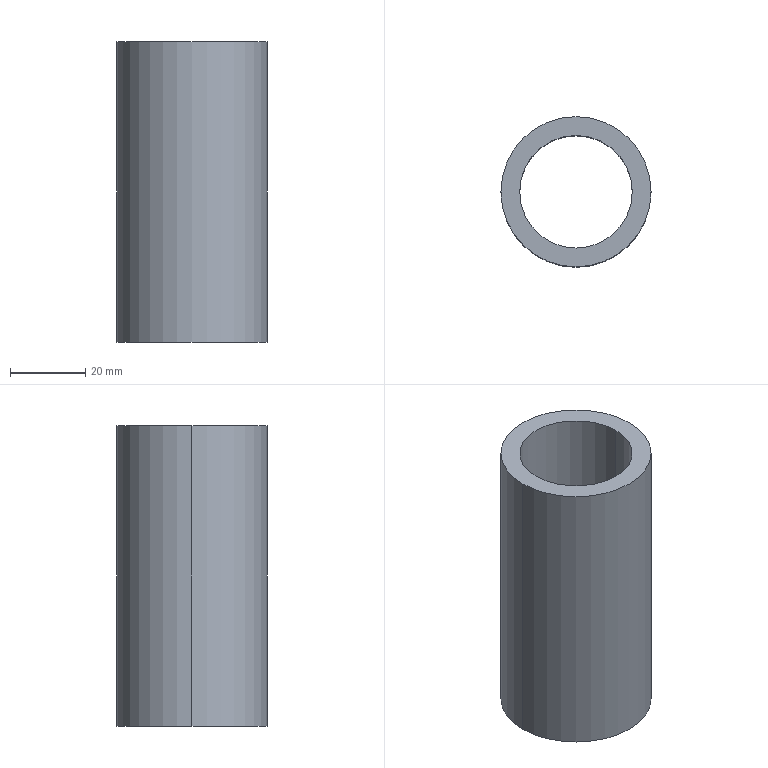Part | SolidWorks | 1 solid | 6 faces | box 40 x 40 x 80 mm | volume 43982 mm3 | cylinder 4 | plane 2 | commonest cylinder face diameters 30 x2 40 x2
STEP:
#1=CARTESIAN_POINT('',(175.,270.,40.));
#2=VERTEX_POINT('',#1);
#3=CARTESIAN_POINT('',(205.,270.,40.));
#4=VERTEX_POINT('',#3);
#5=CARTESIAN_POINT('',(190.,270.,40.));
#6=DIRECTION('',(0.,0.,1.));
#7=DIRECTION('',(1.,0.,0.));
#8=AXIS2_PLACEMENT_3D('',#5,#6,#7);
#9=CIRCLE('',#8,15.);
#10=EDGE_CURVE('',#2,#4,#9,.T.);
#11=ORIENTED_EDGE('',*,*,#10,.T.);
#12=CARTESIAN_POINT('',(205.,270.,-40.));
#13=VERTEX_POINT('',#12);
#14=CARTESIAN_POINT('',(205.,270.,40.));
#15=DIRECTION('',(0.,0.,-1.));
#16=VECTOR('',#15,1000.);
#17=LINE('',#14,#16);
#18=EDGE_CURVE('',#4,#13,#17,.T.);
#19=ORIENTED_EDGE('',*,*,#18,.T.);
#20=CARTESIAN_POINT('',(175.,270.,-40.));
#21=VERTEX_POINT('',#20);
#22=CARTESIAN_POINT('',(190.,270.,-40.));
#23=DIRECTION('',(0.,0.,1.));
#24=DIRECTION('',(1.,0.,0.));
#25=AXIS2_PLACEMENT_3D('',#22,#23,#24);
#26=CIRCLE('',#25,15.);
#27=EDGE_CURVE('',#21,#13,#26,.T.);
#28=ORIENTED_EDGE('',*,*,#27,.F.);
#29=CARTESIAN_POINT('',(175.,270.,40.));
#30=DIRECTION('',(0.,0.,-1.));
#31=VECTOR('',#30,1000.);
#32=LINE('',#29,#31);
#33=EDGE_CURVE('',#2,#21,#32,.T.);
#34=ORIENTED_EDGE('',*,*,#33,.F.);
#35=EDGE_LOOP('',(#11,#19,#28,#34));
#36=FACE_OUTER_BOUND('',#35,.T.);
#37=CARTESIAN_POINT('',(190.,270.,40.));
#38=DIRECTION('',(0.,0.,-1.));
#39=DIRECTION('',(-1.,0.,0.));
#40=AXIS2_PLACEMENT_3D('',#37,#38,#39);
#41=CYLINDRICAL_SURFACE('',#40,15.);
#42=ADVANCED_FACE('',(#36),#41,.F.);
#43=CARTESIAN_POINT('',(210.,270.,40.));
#44=VERTEX_POINT('',#43);
#45=CARTESIAN_POINT('',(170.,270.,40.));
#46=VERTEX_POINT('',#45);
#47=CARTESIAN_POINT('',(190.,270.,40.));
#48=DIRECTION('',(0.,0.,1.));
#49=DIRECTION('',(1.,0.,0.));
#50=AXIS2_PLACEMENT_3D('',#47,#48,#49);
#51=CIRCLE('',#50,20.);
#52=EDGE_CURVE('',#44,#46,#51,.T.);
#53=ORIENTED_EDGE('',*,*,#52,.F.);
#54=CARTESIAN_POINT('',(210.,270.,-40.));
#55=VERTEX_POINT('',#54);
#56=CARTESIAN_POINT('',(210.,270.,40.));
#57=DIRECTION('',(0.,0.,-1.));
#58=VECTOR('',#57,1000.);
#59=LINE('',#56,#58);
#60=EDGE_CURVE('',#44,#55,#59,.T.);
#61=ORIENTED_EDGE('',*,*,#60,.T.);
#62=CARTESIAN_POINT('',(170.,270.,-40.));
#63=VERTEX_POINT('',#62);
#64=CARTESIAN_POINT('',(190.,270.,-40.));
#65=DIRECTION('',(0.,0.,1.));
#66=DIRECTION('',(1.,0.,0.));
#67=AXIS2_PLACEMENT_3D('',#64,#65,#66);
#68=CIRCLE('',#67,20.);
#69=EDGE_CURVE('',#55,#63,#68,.T.);
#70=ORIENTED_EDGE('',*,*,#69,.T.);
#71=CARTESIAN_POINT('',(170.,270.,40.));
#72=DIRECTION('',(0.,0.,-1.));
#73=VECTOR('',#72,1000.);
#74=LINE('',#71,#73);
#75=EDGE_CURVE('',#46,#63,#74,.T.);
#76=ORIENTED_EDGE('',*,*,#75,.F.);
#77=EDGE_LOOP('',(#53,#61,#70,#76));
#78=FACE_OUTER_BOUND('',#77,.T.);
#79=CARTESIAN_POINT('',(190.,270.,40.));
#80=DIRECTION('',(0.,0.,-1.));
#81=DIRECTION('',(-1.,0.,0.));
#82=AXIS2_PLACEMENT_3D('',#79,#80,#81);
#83=CYLINDRICAL_SURFACE('',#82,20.);
#84=ADVANCED_FACE('',(#78),#83,.T.);
#85=CARTESIAN_POINT('',(190.,270.,40.));
#86=DIRECTION('',(0.,0.,1.));
#87=DIRECTION('',(1.,0.,0.));
#88=AXIS2_PLACEMENT_3D('',#85,#86,#87);
#89=CIRCLE('',#88,20.);
#90=EDGE_CURVE('',#46,#44,#89,.T.);
#91=ORIENTED_EDGE('',*,*,#90,.T.);
#92=ORIENTED_EDGE('',*,*,#52,.T.);
#93=EDGE_LOOP('',(#91,#92));
#94=FACE_OUTER_BOUND('',#93,.T.);
#95=ORIENTED_EDGE('',*,*,#10,.F.);
#96=CARTESIAN_POINT('',(190.,270.,40.));
#97=DIRECTION('',(0.,0.,1.));
#98=DIRECTION('',(1.,0.,0.));
#99=AXIS2_PLACEMENT_3D('',#96,#97,#98);
#100=CIRCLE('',#99,15.);
#101=EDGE_CURVE('',#4,#2,#100,.T.);
#102=ORIENTED_EDGE('',*,*,#101,.F.);
#103=EDGE_LOOP('',(#95,#102));
#104=FACE_BOUND('',#103,.T.);
#105=CARTESIAN_POINT('',(190.,270.,40.));
#106=DIRECTION('',(0.,0.,1.));
#107=DIRECTION('',(1.,0.,0.));
#108=AXIS2_PLACEMENT_3D('',#105,#106,#107);
#109=PLANE('',#108);
#110=ADVANCED_FACE('',(#94,#104),#109,.T.);
#111=CARTESIAN_POINT('',(190.,270.,-40.));
#112=DIRECTION('',(0.,0.,1.));
#113=DIRECTION('',(1.,0.,0.));
#114=AXIS2_PLACEMENT_3D('',#111,#112,#113);
#115=CIRCLE('',#114,20.);
#116=EDGE_CURVE('',#63,#55,#115,.T.);
#117=ORIENTED_EDGE('',*,*,#116,.F.);
#118=ORIENTED_EDGE('',*,*,#69,.F.);
#119=EDGE_LOOP('',(#117,#118));
#120=FACE_OUTER_BOUND('',#119,.T.);
#121=ORIENTED_EDGE('',*,*,#27,.T.);
#122=CARTESIAN_POINT('',(190.,270.,-40.));
#123=DIRECTION('',(0.,0.,1.));
#124=DIRECTION('',(1.,0.,0.));
#125=AXIS2_PLACEMENT_3D('',#122,#123,#124);
#126=CIRCLE('',#125,15.);
#127=EDGE_CURVE('',#13,#21,#126,.T.);
#128=ORIENTED_EDGE('',*,*,#127,.T.);
#129=EDGE_LOOP('',(#121,#128));
#130=FACE_BOUND('',#129,.T.);
#131=CARTESIAN_POINT('',(190.,270.,-40.));
#132=DIRECTION('',(0.,0.,1.));
#133=DIRECTION('',(1.,0.,0.));
#134=AXIS2_PLACEMENT_3D('',#131,#132,#133);
#135=PLANE('',#134);
#136=ADVANCED_FACE('',(#120,#130),#135,.F.);
#137=ORIENTED_EDGE('',*,*,#60,.F.);
#138=ORIENTED_EDGE('',*,*,#90,.F.);
#139=ORIENTED_EDGE('',*,*,#75,.T.);
#140=ORIENTED_EDGE('',*,*,#116,.T.);
#141=EDGE_LOOP('',(#137,#138,#139,#140));
#142=FACE_OUTER_BOUND('',#141,.T.);
#143=CARTESIAN_POINT('',(190.,270.,40.));
#144=DIRECTION('',(0.,0.,-1.));
#145=DIRECTION('',(-1.,0.,0.));
#146=AXIS2_PLACEMENT_3D('',#143,#144,#145);
#147=CYLINDRICAL_SURFACE('',#146,20.);
#148=ADVANCED_FACE('',(#142),#147,.T.);
#149=ORIENTED_EDGE('',*,*,#18,.F.);
#150=ORIENTED_EDGE('',*,*,#101,.T.);
#151=ORIENTED_EDGE('',*,*,#33,.T.);
#152=ORIENTED_EDGE('',*,*,#127,.F.);
#153=EDGE_LOOP('',(#149,#150,#151,#152));
#154=FACE_OUTER_BOUND('',#153,.T.);
#155=CARTESIAN_POINT('',(190.,270.,40.));
#156=DIRECTION('',(0.,0.,-1.));
#157=DIRECTION('',(-1.,0.,0.));
#158=AXIS2_PLACEMENT_3D('',#155,#156,#157);
#159=CYLINDRICAL_SURFACE('',#158,15.);
#160=ADVANCED_FACE('',(#154),#159,.F.);
#161=CLOSED_SHELL('',(#42,#84,#110,#136,#148,#160));
#162=MANIFOLD_SOLID_BREP('',#161);
#163=CARTESIAN_POINT('',(0.,0.,0.));
#164=DIRECTION('',(0.,0.,1.));
#165=DIRECTION('',(1.,0.,0.));
#166=AXIS2_PLACEMENT_3D('',#163,#164,#165);
#167=(LENGTH_UNIT()NAMED_UNIT(*)SI_UNIT(.MILLI.,.METRE.));
#168=UNCERTAINTY_MEASURE_WITH_UNIT(LENGTH_MEASURE(0.00001),#167,'','');
#169=(NAMED_UNIT(*)PLANE_ANGLE_UNIT()SI_UNIT($,.RADIAN.));
#170=(NAMED_UNIT(*)SI_UNIT($,.STERADIAN.)SOLID_ANGLE_UNIT());
#171=(GEOMETRIC_REPRESENTATION_CONTEXT(3)GLOBAL_UNCERTAINTY_ASSIGNED_CONTEXT((#168))GLOBAL_UNIT_ASSIGNED_CONTEXT((#167,#169,#170))REPRESENTATION_CONTEXT('',''));
#172=ADVANCED_BREP_SHAPE_REPRESENTATION('',(#162,#166),#171);